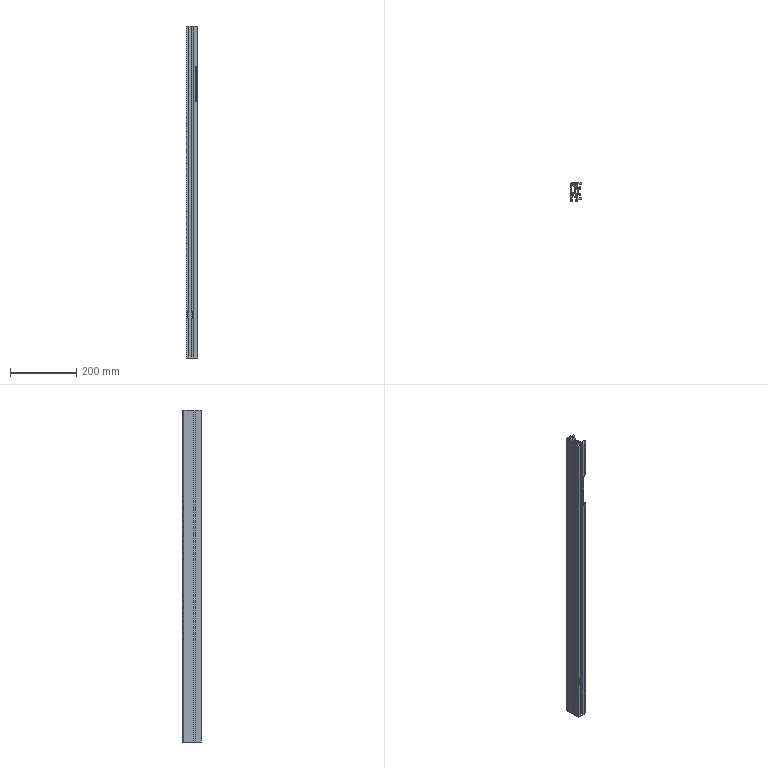Part | STEP file | 1 solid | 182 faces | box 35 x 55 x 1000 mm | volume 772686 mm3 | plane 132 | cylinder 41 | cone 9 | commonest cylinder face diameters 2.5 x9 2 x8 6.5 x6 2.3 x4 11 x4 13 x4